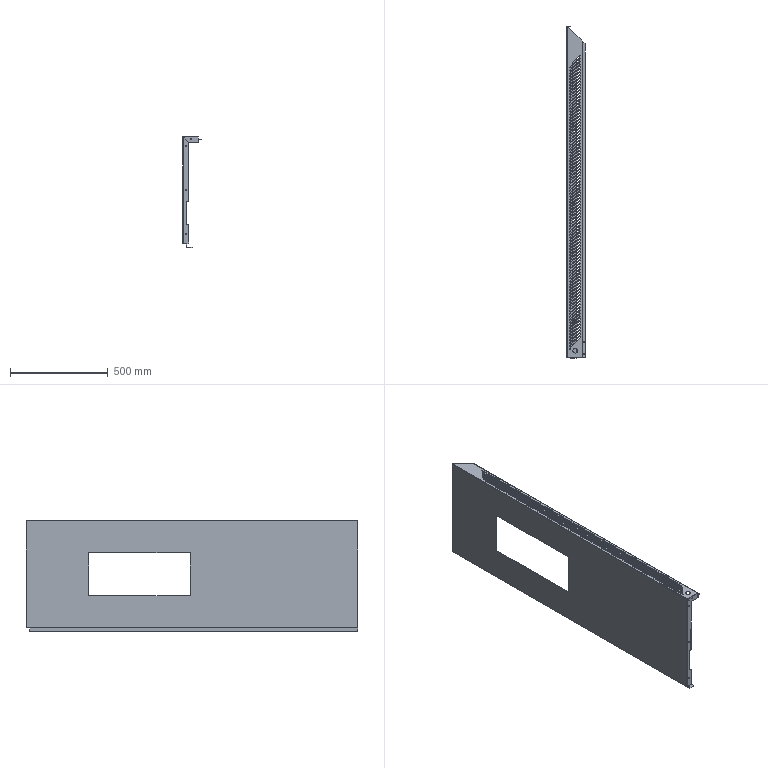Part | STEP file | HESS-408-70-15W-D-1-electrical box left side panel | 1 solid | 633 faces | box 93.5 x 1699 x 568.5 mm | volume 1630922 mm3 | cylinder 366 | plane 261 | spline 6 | commonest cylinder face diameters 5 x291 3.2 x15 5.5 x14 6 x11 0.2 x9 15 x9